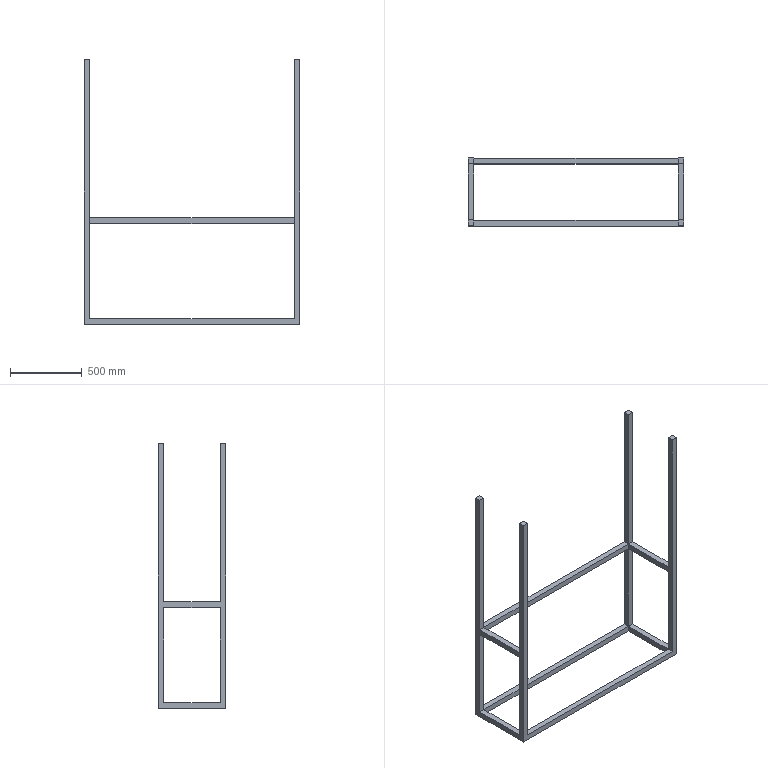Part | STEP file | Upper frame | 1 solid | 38 faces | box 1500 x 470 x 1840 mm | volume 21088000 mm3 | plane 38